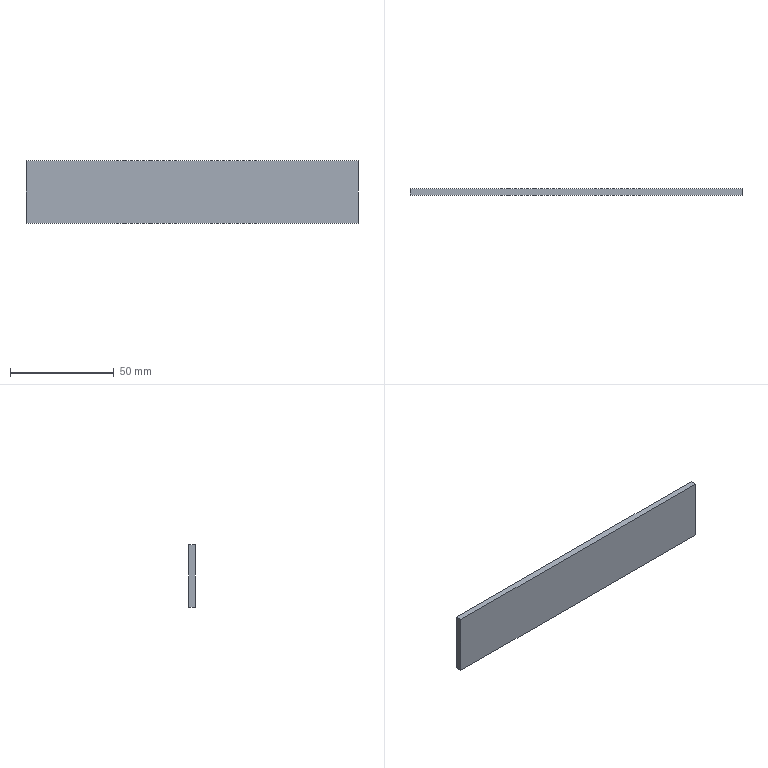Part | NX | features BREP 1 | 1 solid | 6 faces | box 160 x 3 x 30 mm | volume 14400 mm3 | plane 6
STEP:
#1=CARTESIAN_POINT('',(-80.,0.,15.));
#2=VERTEX_POINT('',#1);
#3=CARTESIAN_POINT('',(80.,0.,15.));
#4=VERTEX_POINT('',#3);
#5=CARTESIAN_POINT('',(0.,0.,15.));
#6=DIRECTION('',(1.,0.,0.));
#7=VECTOR('',#6,1000.);
#8=LINE('',#5,#7);
#9=EDGE_CURVE('',#2,#4,#8,.T.);
#10=ORIENTED_EDGE('',*,*,#9,.F.);
#11=CARTESIAN_POINT('',(-80.,0.,-15.));
#12=VERTEX_POINT('',#11);
#13=CARTESIAN_POINT('',(-80.,0.,0.));
#14=DIRECTION('',(0.,0.,1.));
#15=VECTOR('',#14,1000.);
#16=LINE('',#13,#15);
#17=EDGE_CURVE('',#12,#2,#16,.T.);
#18=ORIENTED_EDGE('',*,*,#17,.F.);
#19=CARTESIAN_POINT('',(80.,0.,-15.));
#20=VERTEX_POINT('',#19);
#21=CARTESIAN_POINT('',(0.,0.,-15.));
#22=DIRECTION('',(-1.,0.,0.));
#23=VECTOR('',#22,1000.);
#24=LINE('',#21,#23);
#25=EDGE_CURVE('',#20,#12,#24,.T.);
#26=ORIENTED_EDGE('',*,*,#25,.F.);
#27=CARTESIAN_POINT('',(80.,0.,0.));
#28=DIRECTION('',(0.,0.,-1.));
#29=VECTOR('',#28,1000.);
#30=LINE('',#27,#29);
#31=EDGE_CURVE('',#4,#20,#30,.T.);
#32=ORIENTED_EDGE('',*,*,#31,.F.);
#33=EDGE_LOOP('',(#10,#18,#26,#32));
#34=FACE_BOUND('',#33,.T.);
#35=CARTESIAN_POINT('',(0.,0.,0.));
#36=DIRECTION('',(0.,1.,0.));
#37=DIRECTION('',(0.,0.,-1.));
#38=AXIS2_PLACEMENT_3D('',#35,#36,#37);
#39=PLANE('',#38);
#40=ADVANCED_FACE('',(#34),#39,.F.);
#41=CARTESIAN_POINT('',(80.,3.,-15.));
#42=VERTEX_POINT('',#41);
#43=CARTESIAN_POINT('',(80.,0.,-15.));
#44=DIRECTION('',(0.,1.,0.));
#45=VECTOR('',#44,1000.);
#46=LINE('',#43,#45);
#47=EDGE_CURVE('',#20,#42,#46,.T.);
#48=ORIENTED_EDGE('',*,*,#47,.T.);
#49=CARTESIAN_POINT('',(80.,3.,15.));
#50=VERTEX_POINT('',#49);
#51=CARTESIAN_POINT('',(80.,3.,15.));
#52=DIRECTION('',(0.,0.,1.));
#53=VECTOR('',#52,1000.);
#54=LINE('',#51,#53);
#55=EDGE_CURVE('',#42,#50,#54,.T.);
#56=ORIENTED_EDGE('',*,*,#55,.T.);
#57=CARTESIAN_POINT('',(80.,0.,15.));
#58=DIRECTION('',(0.,-1.,0.));
#59=VECTOR('',#58,1000.);
#60=LINE('',#57,#59);
#61=EDGE_CURVE('',#50,#4,#60,.T.);
#62=ORIENTED_EDGE('',*,*,#61,.T.);
#63=ORIENTED_EDGE('',*,*,#31,.T.);
#64=EDGE_LOOP('',(#48,#56,#62,#63));
#65=FACE_BOUND('',#64,.T.);
#66=CARTESIAN_POINT('',(80.,0.,15.));
#67=DIRECTION('',(1.,0.,0.));
#68=DIRECTION('',(0.,0.,1.));
#69=AXIS2_PLACEMENT_3D('',#66,#67,#68);
#70=PLANE('',#69);
#71=ADVANCED_FACE('',(#65),#70,.T.);
#72=ORIENTED_EDGE('',*,*,#61,.F.);
#73=CARTESIAN_POINT('',(-80.,3.,15.));
#74=VERTEX_POINT('',#73);
#75=CARTESIAN_POINT('',(-80.,3.,15.));
#76=DIRECTION('',(-1.,0.,0.));
#77=VECTOR('',#76,1000.);
#78=LINE('',#75,#77);
#79=EDGE_CURVE('',#50,#74,#78,.T.);
#80=ORIENTED_EDGE('',*,*,#79,.T.);
#81=CARTESIAN_POINT('',(-80.,0.,15.));
#82=DIRECTION('',(0.,-1.,0.));
#83=VECTOR('',#82,1000.);
#84=LINE('',#81,#83);
#85=EDGE_CURVE('',#74,#2,#84,.T.);
#86=ORIENTED_EDGE('',*,*,#85,.T.);
#87=ORIENTED_EDGE('',*,*,#9,.T.);
#88=EDGE_LOOP('',(#72,#80,#86,#87));
#89=FACE_BOUND('',#88,.T.);
#90=CARTESIAN_POINT('',(-80.,0.,15.));
#91=DIRECTION('',(0.,0.,1.));
#92=DIRECTION('',(-1.,0.,0.));
#93=AXIS2_PLACEMENT_3D('',#90,#91,#92);
#94=PLANE('',#93);
#95=ADVANCED_FACE('',(#89),#94,.T.);
#96=ORIENTED_EDGE('',*,*,#85,.F.);
#97=CARTESIAN_POINT('',(-80.,3.,-15.));
#98=VERTEX_POINT('',#97);
#99=CARTESIAN_POINT('',(-80.,3.,-15.));
#100=DIRECTION('',(0.,0.,-1.));
#101=VECTOR('',#100,1000.);
#102=LINE('',#99,#101);
#103=EDGE_CURVE('',#74,#98,#102,.T.);
#104=ORIENTED_EDGE('',*,*,#103,.T.);
#105=CARTESIAN_POINT('',(-80.,0.,-15.));
#106=DIRECTION('',(0.,-1.,0.));
#107=VECTOR('',#106,1000.);
#108=LINE('',#105,#107);
#109=EDGE_CURVE('',#98,#12,#108,.T.);
#110=ORIENTED_EDGE('',*,*,#109,.T.);
#111=ORIENTED_EDGE('',*,*,#17,.T.);
#112=EDGE_LOOP('',(#96,#104,#110,#111));
#113=FACE_BOUND('',#112,.T.);
#114=CARTESIAN_POINT('',(-80.,0.,-15.));
#115=DIRECTION('',(-1.,0.,0.));
#116=DIRECTION('',(0.,0.,-1.));
#117=AXIS2_PLACEMENT_3D('',#114,#115,#116);
#118=PLANE('',#117);
#119=ADVANCED_FACE('',(#113),#118,.T.);
#120=ORIENTED_EDGE('',*,*,#109,.F.);
#121=CARTESIAN_POINT('',(80.,3.,-15.));
#122=DIRECTION('',(1.,0.,0.));
#123=VECTOR('',#122,1000.);
#124=LINE('',#121,#123);
#125=EDGE_CURVE('',#98,#42,#124,.T.);
#126=ORIENTED_EDGE('',*,*,#125,.T.);
#127=ORIENTED_EDGE('',*,*,#47,.F.);
#128=ORIENTED_EDGE('',*,*,#25,.T.);
#129=EDGE_LOOP('',(#120,#126,#127,#128));
#130=FACE_BOUND('',#129,.T.);
#131=CARTESIAN_POINT('',(80.,0.,-15.));
#132=DIRECTION('',(0.,0.,-1.));
#133=DIRECTION('',(1.,0.,0.));
#134=AXIS2_PLACEMENT_3D('',#131,#132,#133);
#135=PLANE('',#134);
#136=ADVANCED_FACE('',(#130),#135,.T.);
#137=ORIENTED_EDGE('',*,*,#79,.F.);
#138=ORIENTED_EDGE('',*,*,#55,.F.);
#139=ORIENTED_EDGE('',*,*,#125,.F.);
#140=ORIENTED_EDGE('',*,*,#103,.F.);
#141=EDGE_LOOP('',(#137,#138,#139,#140));
#142=FACE_BOUND('',#141,.T.);
#143=CARTESIAN_POINT('',(0.,3.,0.));
#144=DIRECTION('',(0.,1.,0.));
#145=DIRECTION('',(0.,0.,-1.));
#146=AXIS2_PLACEMENT_3D('',#143,#144,#145);
#147=PLANE('',#146);
#148=ADVANCED_FACE('',(#142),#147,.T.);
#149=CLOSED_SHELL('',(#40,#71,#95,#119,#136,#148));
#150=MANIFOLD_SOLID_BREP('',#149);
#151=(LENGTH_UNIT()NAMED_UNIT(*)SI_UNIT(.MILLI.,.METRE.));
#152=UNCERTAINTY_MEASURE_WITH_UNIT(LENGTH_MEASURE(0.00001),#151,'','');
#153=(NAMED_UNIT(*)PLANE_ANGLE_UNIT()SI_UNIT($,.RADIAN.));
#154=(NAMED_UNIT(*)SI_UNIT($,.STERADIAN.)SOLID_ANGLE_UNIT());
#155=(GEOMETRIC_REPRESENTATION_CONTEXT(3)GLOBAL_UNCERTAINTY_ASSIGNED_CONTEXT((#152))GLOBAL_UNIT_ASSIGNED_CONTEXT((#151,#153,#154))REPRESENTATION_CONTEXT('',''));
#156=ADVANCED_BREP_SHAPE_REPRESENTATION('',(#150),#155);